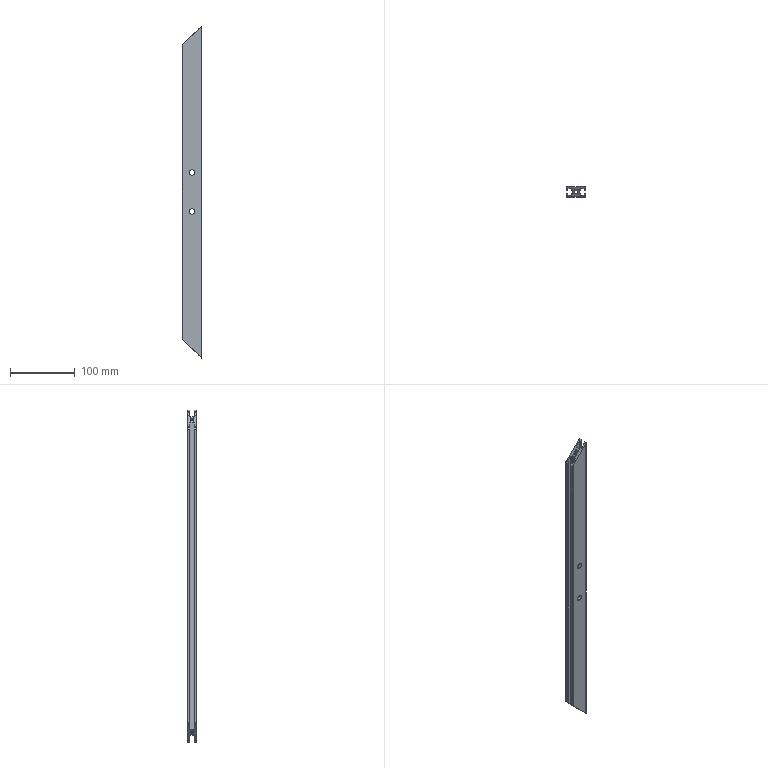Part | NX | features BREP 1 | 1 solid | 95 faces | box 30 x 15 x 512.1 mm | volume 114959 mm3 | plane 54 | cylinder 41 | commonest cylinder face diameters 1 x18 5 x15 2 x4 8.5 x4